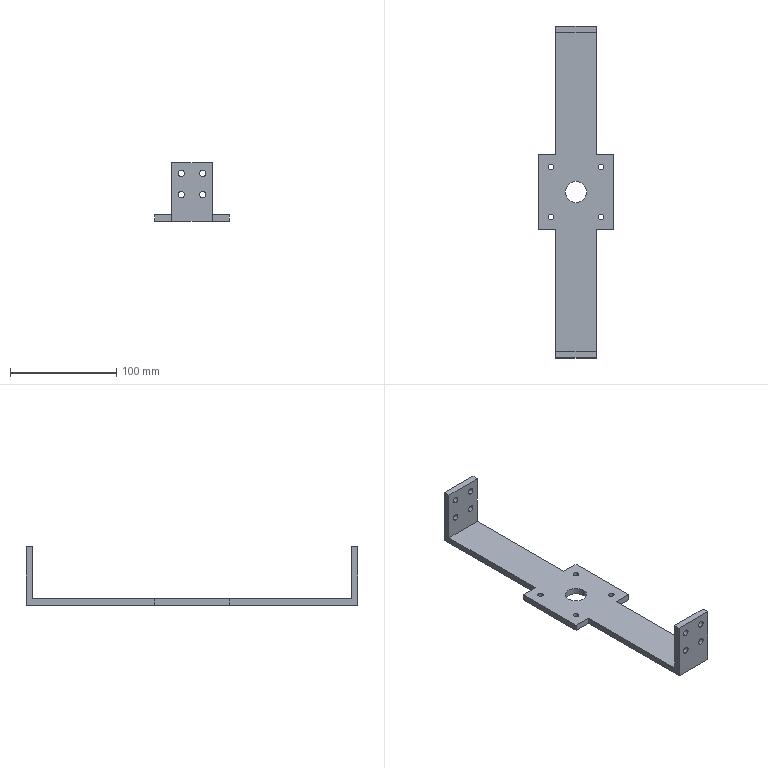Part | SolidWorks | features ICE 4, Cut 1, Extrusion 1 | 1 solid | 44 faces | box 70 x 312 x 55 mm | volume 103168 mm3 | cylinder 26 | plane 18 | commonest cylinder face diameters 6 x16 5.2 x8 20 x2
STEP:
#1=CARTESIAN_POINT('',(10.,156.,-21.5));
#2=VERTEX_POINT('',#1);
#3=CARTESIAN_POINT('',(-10.,156.,-21.5));
#4=VERTEX_POINT('',#3);
#5=CARTESIAN_POINT('',(0.,156.,-21.5));
#6=DIRECTION('',(0.,0.,-1.));
#7=DIRECTION('',(-1.,0.,0.));
#8=AXIS2_PLACEMENT_3D('',#5,#6,#7);
#9=CIRCLE('',#8,10.);
#10=EDGE_CURVE('',#2,#4,#9,.T.);
#11=ORIENTED_EDGE('',*,*,#10,.F.);
#12=CARTESIAN_POINT('',(10.,156.,-27.5));
#13=VERTEX_POINT('',#12);
#14=CARTESIAN_POINT('',(10.,156.,-17.5));
#15=DIRECTION('',(0.,0.,-1.));
#16=VECTOR('',#15,1000.);
#17=LINE('',#14,#16);
#18=EDGE_CURVE('',#2,#13,#17,.T.);
#19=ORIENTED_EDGE('',*,*,#18,.T.);
#20=CARTESIAN_POINT('',(-10.,156.,-27.5));
#21=VERTEX_POINT('',#20);
#22=CARTESIAN_POINT('',(0.,156.,-27.5));
#23=DIRECTION('',(0.,0.,-1.));
#24=DIRECTION('',(-1.,0.,0.));
#25=AXIS2_PLACEMENT_3D('',#22,#23,#24);
#26=CIRCLE('',#25,10.);
#27=EDGE_CURVE('',#13,#21,#26,.T.);
#28=ORIENTED_EDGE('',*,*,#27,.T.);
#29=CARTESIAN_POINT('',(-10.,156.,-17.5));
#30=DIRECTION('',(0.,0.,-1.));
#31=VECTOR('',#30,1000.);
#32=LINE('',#29,#31);
#33=EDGE_CURVE('',#4,#21,#32,.T.);
#34=ORIENTED_EDGE('',*,*,#33,.F.);
#35=EDGE_LOOP('',(#11,#19,#28,#34));
#36=FACE_OUTER_BOUND('',#35,.T.);
#37=CARTESIAN_POINT('',(0.,156.,-17.5));
#38=DIRECTION('',(0.,0.,-1.));
#39=DIRECTION('',(-1.,0.,0.));
#40=AXIS2_PLACEMENT_3D('',#37,#38,#39);
#41=CYLINDRICAL_SURFACE('',#40,10.);
#42=ADVANCED_FACE('',(#36),#41,.F.);
#43=CARTESIAN_POINT('',(26.145,179.545,-21.5));
#44=VERTEX_POINT('',#43);
#45=CARTESIAN_POINT('',(20.945,179.545,-21.5));
#46=VERTEX_POINT('',#45);
#47=CARTESIAN_POINT('',(23.545,179.545,-21.5));
#48=DIRECTION('',(0.,0.,-1.));
#49=DIRECTION('',(-1.,0.,0.));
#50=AXIS2_PLACEMENT_3D('',#47,#48,#49);
#51=CIRCLE('',#50,2.6);
#52=EDGE_CURVE('',#44,#46,#51,.T.);
#53=ORIENTED_EDGE('',*,*,#52,.F.);
#54=CARTESIAN_POINT('',(26.145,179.545,-27.5));
#55=VERTEX_POINT('',#54);
#56=CARTESIAN_POINT('',(26.145,179.545,-17.5));
#57=DIRECTION('',(0.,0.,-1.));
#58=VECTOR('',#57,1000.);
#59=LINE('',#56,#58);
#60=EDGE_CURVE('',#44,#55,#59,.T.);
#61=ORIENTED_EDGE('',*,*,#60,.T.);
#62=CARTESIAN_POINT('',(20.945,179.545,-27.5));
#63=VERTEX_POINT('',#62);
#64=CARTESIAN_POINT('',(23.545,179.545,-27.5));
#65=DIRECTION('',(0.,0.,-1.));
#66=DIRECTION('',(-1.,0.,0.));
#67=AXIS2_PLACEMENT_3D('',#64,#65,#66);
#68=CIRCLE('',#67,2.6);
#69=EDGE_CURVE('',#55,#63,#68,.T.);
#70=ORIENTED_EDGE('',*,*,#69,.T.);
#71=CARTESIAN_POINT('',(20.945,179.545,-17.5));
#72=DIRECTION('',(0.,0.,-1.));
#73=VECTOR('',#72,1000.);
#74=LINE('',#71,#73);
#75=EDGE_CURVE('',#46,#63,#74,.T.);
#76=ORIENTED_EDGE('',*,*,#75,.F.);
#77=EDGE_LOOP('',(#53,#61,#70,#76));
#78=FACE_OUTER_BOUND('',#77,.T.);
#79=CARTESIAN_POINT('',(23.545,179.545,-17.5));
#80=DIRECTION('',(0.,0.,-1.));
#81=DIRECTION('',(-1.,0.,0.));
#82=AXIS2_PLACEMENT_3D('',#79,#80,#81);
#83=CYLINDRICAL_SURFACE('',#82,2.6);
#84=ADVANCED_FACE('',(#78),#83,.F.);
#85=CARTESIAN_POINT('',(26.1,132.5,-21.5));
#86=VERTEX_POINT('',#85);
#87=CARTESIAN_POINT('',(20.9,132.5,-21.5));
#88=VERTEX_POINT('',#87);
#89=CARTESIAN_POINT('',(23.5,132.5,-21.5));
#90=DIRECTION('',(0.,0.,-1.));
#91=DIRECTION('',(-1.,0.,0.));
#92=AXIS2_PLACEMENT_3D('',#89,#90,#91);
#93=CIRCLE('',#92,2.6);
#94=EDGE_CURVE('',#86,#88,#93,.T.);
#95=ORIENTED_EDGE('',*,*,#94,.F.);
#96=CARTESIAN_POINT('',(26.1,132.5,-27.5));
#97=VERTEX_POINT('',#96);
#98=CARTESIAN_POINT('',(26.1,132.5,-17.5));
#99=DIRECTION('',(0.,0.,-1.));
#100=VECTOR('',#99,1000.);
#101=LINE('',#98,#100);
#102=EDGE_CURVE('',#86,#97,#101,.T.);
#103=ORIENTED_EDGE('',*,*,#102,.T.);
#104=CARTESIAN_POINT('',(20.9,132.5,-27.5));
#105=VERTEX_POINT('',#104);
#106=CARTESIAN_POINT('',(23.5,132.5,-27.5));
#107=DIRECTION('',(0.,0.,-1.));
#108=DIRECTION('',(-1.,0.,0.));
#109=AXIS2_PLACEMENT_3D('',#106,#107,#108);
#110=CIRCLE('',#109,2.6);
#111=EDGE_CURVE('',#97,#105,#110,.T.);
#112=ORIENTED_EDGE('',*,*,#111,.T.);
#113=CARTESIAN_POINT('',(20.9,132.5,-17.5));
#114=DIRECTION('',(0.,0.,-1.));
#115=VECTOR('',#114,1000.);
#116=LINE('',#113,#115);
#117=EDGE_CURVE('',#88,#105,#116,.T.);
#118=ORIENTED_EDGE('',*,*,#117,.F.);
#119=EDGE_LOOP('',(#95,#103,#112,#118));
#120=FACE_OUTER_BOUND('',#119,.T.);
#121=CARTESIAN_POINT('',(23.5,132.5,-17.5));
#122=DIRECTION('',(0.,0.,-1.));
#123=DIRECTION('',(-1.,0.,0.));
#124=AXIS2_PLACEMENT_3D('',#121,#122,#123);
#125=CYLINDRICAL_SURFACE('',#124,2.6);
#126=ADVANCED_FACE('',(#120),#125,.F.);
#127=CARTESIAN_POINT('',(-20.9,132.5,-21.5));
#128=VERTEX_POINT('',#127);
#129=CARTESIAN_POINT('',(-26.1,132.5,-21.5));
#130=VERTEX_POINT('',#129);
#131=CARTESIAN_POINT('',(-23.5,132.5,-21.5));
#132=DIRECTION('',(0.,0.,-1.));
#133=DIRECTION('',(-1.,0.,0.));
#134=AXIS2_PLACEMENT_3D('',#131,#132,#133);
#135=CIRCLE('',#134,2.6);
#136=EDGE_CURVE('',#128,#130,#135,.T.);
#137=ORIENTED_EDGE('',*,*,#136,.F.);
#138=CARTESIAN_POINT('',(-20.9,132.5,-27.5));
#139=VERTEX_POINT('',#138);
#140=CARTESIAN_POINT('',(-20.9,132.5,-17.5));
#141=DIRECTION('',(0.,0.,-1.));
#142=VECTOR('',#141,1000.);
#143=LINE('',#140,#142);
#144=EDGE_CURVE('',#128,#139,#143,.T.);
#145=ORIENTED_EDGE('',*,*,#144,.T.);
#146=CARTESIAN_POINT('',(-26.1,132.5,-27.5));
#147=VERTEX_POINT('',#146);
#148=CARTESIAN_POINT('',(-23.5,132.5,-27.5));
#149=DIRECTION('',(0.,0.,-1.));
#150=DIRECTION('',(-1.,0.,0.));
#151=AXIS2_PLACEMENT_3D('',#148,#149,#150);
#152=CIRCLE('',#151,2.6);
#153=EDGE_CURVE('',#139,#147,#152,.T.);
#154=ORIENTED_EDGE('',*,*,#153,.T.);
#155=CARTESIAN_POINT('',(-26.1,132.5,-17.5));
#156=DIRECTION('',(0.,0.,-1.));
#157=VECTOR('',#156,1000.);
#158=LINE('',#155,#157);
#159=EDGE_CURVE('',#130,#147,#158,.T.);
#160=ORIENTED_EDGE('',*,*,#159,.F.);
#161=EDGE_LOOP('',(#137,#145,#154,#160));
#162=FACE_OUTER_BOUND('',#161,.T.);
#163=CARTESIAN_POINT('',(-23.5,132.5,-17.5));
#164=DIRECTION('',(0.,0.,-1.));
#165=DIRECTION('',(-1.,0.,0.));
#166=AXIS2_PLACEMENT_3D('',#163,#164,#165);
#167=CYLINDRICAL_SURFACE('',#166,2.6);
#168=ADVANCED_FACE('',(#162),#167,.F.);
#169=CARTESIAN_POINT('',(-20.945,179.545,-21.5));
#170=VERTEX_POINT('',#169);
#171=CARTESIAN_POINT('',(-26.145,179.545,-21.5));
#172=VERTEX_POINT('',#171);
#173=CARTESIAN_POINT('',(-23.545,179.545,-21.5));
#174=DIRECTION('',(0.,0.,-1.));
#175=DIRECTION('',(-1.,0.,0.));
#176=AXIS2_PLACEMENT_3D('',#173,#174,#175);
#177=CIRCLE('',#176,2.6);
#178=EDGE_CURVE('',#170,#172,#177,.T.);
#179=ORIENTED_EDGE('',*,*,#178,.F.);
#180=CARTESIAN_POINT('',(-20.945,179.545,-27.5));
#181=VERTEX_POINT('',#180);
#182=CARTESIAN_POINT('',(-20.945,179.545,-17.5));
#183=DIRECTION('',(0.,0.,-1.));
#184=VECTOR('',#183,1000.);
#185=LINE('',#182,#184);
#186=EDGE_CURVE('',#170,#181,#185,.T.);
#187=ORIENTED_EDGE('',*,*,#186,.T.);
#188=CARTESIAN_POINT('',(-26.145,179.545,-27.5));
#189=VERTEX_POINT('',#188);
#190=CARTESIAN_POINT('',(-23.545,179.545,-27.5));
#191=DIRECTION('',(0.,0.,-1.));
#192=DIRECTION('',(-1.,0.,0.));
#193=AXIS2_PLACEMENT_3D('',#190,#191,#192);
#194=CIRCLE('',#193,2.6);
#195=EDGE_CURVE('',#181,#189,#194,.T.);
#196=ORIENTED_EDGE('',*,*,#195,.T.);
#197=CARTESIAN_POINT('',(-26.145,179.545,-17.5));
#198=DIRECTION('',(0.,0.,-1.));
#199=VECTOR('',#198,1000.);
#200=LINE('',#197,#199);
#201=EDGE_CURVE('',#172,#189,#200,.T.);
#202=ORIENTED_EDGE('',*,*,#201,.F.);
#203=EDGE_LOOP('',(#179,#187,#196,#202));
#204=FACE_OUTER_BOUND('',#203,.T.);
#205=CARTESIAN_POINT('',(-23.545,179.545,-17.5));
#206=DIRECTION('',(0.,0.,-1.));
#207=DIRECTION('',(-1.,0.,0.));
#208=AXIS2_PLACEMENT_3D('',#205,#206,#207);
#209=CYLINDRICAL_SURFACE('',#208,2.6);
#210=ADVANCED_FACE('',(#204),#209,.F.);
#211=CARTESIAN_POINT('',(10.,312.,14.5));
#212=VERTEX_POINT('',#211);
#213=CARTESIAN_POINT('',(10.,312.,20.5));
#214=VERTEX_POINT('',#213);
#215=CARTESIAN_POINT('',(10.,312.,17.5));
#216=DIRECTION('',(0.,1.,0.));
#217=DIRECTION('',(0.,0.,1.));
#218=AXIS2_PLACEMENT_3D('',#215,#216,#217);
#219=CIRCLE('',#218,3.);
#220=EDGE_CURVE('',#212,#214,#219,.T.);
#221=ORIENTED_EDGE('',*,*,#220,.T.);
#222=CARTESIAN_POINT('',(10.,306.,20.5));
#223=VERTEX_POINT('',#222);
#224=CARTESIAN_POINT('',(10.,312.,20.5));
#225=DIRECTION('',(0.,-1.,0.));
#226=VECTOR('',#225,1000.);
#227=LINE('',#224,#226);
#228=EDGE_CURVE('',#214,#223,#227,.T.);
#229=ORIENTED_EDGE('',*,*,#228,.T.);
#230=CARTESIAN_POINT('',(10.,306.,14.5));
#231=VERTEX_POINT('',#230);
#232=CARTESIAN_POINT('',(10.,306.,17.5));
#233=DIRECTION('',(0.,1.,0.));
#234=DIRECTION('',(0.,0.,1.));
#235=AXIS2_PLACEMENT_3D('',#232,#233,#234);
#236=CIRCLE('',#235,3.);
#237=EDGE_CURVE('',#231,#223,#236,.T.);
#238=ORIENTED_EDGE('',*,*,#237,.F.);
#239=CARTESIAN_POINT('',(10.,312.,14.5));
#240=DIRECTION('',(0.,-1.,0.));
#241=VECTOR('',#240,1000.);
#242=LINE('',#239,#241);
#243=EDGE_CURVE('',#212,#231,#242,.T.);
#244=ORIENTED_EDGE('',*,*,#243,.F.);
#245=EDGE_LOOP('',(#221,#229,#238,#244));
#246=FACE_OUTER_BOUND('',#245,.T.);
#247=CARTESIAN_POINT('',(10.,312.,17.5));
#248=DIRECTION('',(0.,-1.,0.));
#249=DIRECTION('',(0.,0.,-1.));
#250=AXIS2_PLACEMENT_3D('',#247,#248,#249);
#251=CYLINDRICAL_SURFACE('',#250,3.);
#252=ADVANCED_FACE('',(#246),#251,.F.);
#253=CARTESIAN_POINT('',(-10.,312.,14.5));
#254=VERTEX_POINT('',#253);
#255=CARTESIAN_POINT('',(-10.,312.,20.5));
#256=VERTEX_POINT('',#255);
#257=CARTESIAN_POINT('',(-10.,312.,17.5));
#258=DIRECTION('',(0.,1.,0.));
#259=DIRECTION('',(0.,0.,1.));
#260=AXIS2_PLACEMENT_3D('',#257,#258,#259);
#261=CIRCLE('',#260,3.);
#262=EDGE_CURVE('',#254,#256,#261,.T.);
#263=ORIENTED_EDGE('',*,*,#262,.T.);
#264=CARTESIAN_POINT('',(-10.,306.,20.5));
#265=VERTEX_POINT('',#264);
#266=CARTESIAN_POINT('',(-10.,312.,20.5));
#267=DIRECTION('',(0.,-1.,0.));
#268=VECTOR('',#267,1000.);
#269=LINE('',#266,#268);
#270=EDGE_CURVE('',#256,#265,#269,.T.);
#271=ORIENTED_EDGE('',*,*,#270,.T.);
#272=CARTESIAN_POINT('',(-10.,306.,14.5));
#273=VERTEX_POINT('',#272);
#274=CARTESIAN_POINT('',(-10.,306.,17.5));
#275=DIRECTION('',(0.,1.,0.));
#276=DIRECTION('',(0.,0.,1.));
#277=AXIS2_PLACEMENT_3D('',#274,#275,#276);
#278=CIRCLE('',#277,3.);
#279=EDGE_CURVE('',#273,#265,#278,.T.);
#280=ORIENTED_EDGE('',*,*,#279,.F.);
#281=CARTESIAN_POINT('',(-10.,312.,14.5));
#282=DIRECTION('',(0.,-1.,0.));
#283=VECTOR('',#282,1000.);
#284=LINE('',#281,#283);
#285=EDGE_CURVE('',#254,#273,#284,.T.);
#286=ORIENTED_EDGE('',*,*,#285,.F.);
#287=EDGE_LOOP('',(#263,#271,#280,#286));
#288=FACE_OUTER_BOUND('',#287,.T.);
#289=CARTESIAN_POINT('',(-10.,312.,17.5));
#290=DIRECTION('',(0.,-1.,0.));
#291=DIRECTION('',(0.,0.,-1.));
#292=AXIS2_PLACEMENT_3D('',#289,#290,#291);
#293=CYLINDRICAL_SURFACE('',#292,3.);
#294=ADVANCED_FACE('',(#288),#293,.F.);
#295=CARTESIAN_POINT('',(10.,312.,-5.5));
#296=VERTEX_POINT('',#295);
#297=CARTESIAN_POINT('',(10.,312.,0.5));
#298=VERTEX_POINT('',#297);
#299=CARTESIAN_POINT('',(10.,312.,-2.5));
#300=DIRECTION('',(0.,1.,0.));
#301=DIRECTION('',(0.,0.,1.));
#302=AXIS2_PLACEMENT_3D('',#299,#300,#301);
#303=CIRCLE('',#302,3.);
#304=EDGE_CURVE('',#296,#298,#303,.T.);
#305=ORIENTED_EDGE('',*,*,#304,.T.);
#306=CARTESIAN_POINT('',(10.,306.,0.5));
#307=VERTEX_POINT('',#306);
#308=CARTESIAN_POINT('',(10.,312.,0.5));
#309=DIRECTION('',(0.,-1.,0.));
#310=VECTOR('',#309,1000.);
#311=LINE('',#308,#310);
#312=EDGE_CURVE('',#298,#307,#311,.T.);
#313=ORIENTED_EDGE('',*,*,#312,.T.);
#314=CARTESIAN_POINT('',(10.,306.,-5.5));
#315=VERTEX_POINT('',#314);
#316=CARTESIAN_POINT('',(10.,306.,-2.5));
#317=DIRECTION('',(0.,1.,0.));
#318=DIRECTION('',(0.,0.,1.));
#319=AXIS2_PLACEMENT_3D('',#316,#317,#318);
#320=CIRCLE('',#319,3.);
#321=EDGE_CURVE('',#315,#307,#320,.T.);
#322=ORIENTED_EDGE('',*,*,#321,.F.);
#323=CARTESIAN_POINT('',(10.,312.,-5.5));
#324=DIRECTION('',(0.,-1.,0.));
#325=VECTOR('',#324,1000.);
#326=LINE('',#323,#325);
#327=EDGE_CURVE('',#296,#315,#326,.T.);
#328=ORIENTED_EDGE('',*,*,#327,.F.);
#329=EDGE_LOOP('',(#305,#313,#322,#328));
#330=FACE_OUTER_BOUND('',#329,.T.);
#331=CARTESIAN_POINT('',(10.,312.,-2.5));
#332=DIRECTION('',(0.,-1.,0.));
#333=DIRECTION('',(0.,0.,-1.));
#334=AXIS2_PLACEMENT_3D('',#331,#332,#333);
#335=CYLINDRICAL_SURFACE('',#334,3.);
#336=ADVANCED_FACE('',(#330),#335,.F.);
#337=CARTESIAN_POINT('',(-10.,312.,-5.5));
#338=VERTEX_POINT('',#337);
#339=CARTESIAN_POINT('',(-10.,312.,0.5));
#340=VERTEX_POINT('',#339);
#341=CARTESIAN_POINT('',(-10.,312.,-2.5));
#342=DIRECTION('',(0.,1.,0.));
#343=DIRECTION('',(0.,0.,1.));
#344=AXIS2_PLACEMENT_3D('',#341,#342,#343);
#345=CIRCLE('',#344,3.);
#346=EDGE_CURVE('',#338,#340,#345,.T.);
#347=ORIENTED_EDGE('',*,*,#346,.T.);
#348=CARTESIAN_POINT('',(-10.,306.,0.5));
#349=VERTEX_POINT('',#348);
#350=CARTESIAN_POINT('',(-10.,312.,0.5));
#351=DIRECTION('',(0.,-1.,0.));
#352=VECTOR('',#351,1000.);
#353=LINE('',#350,#352);
#354=EDGE_CURVE('',#340,#349,#353,.T.);
#355=ORIENTED_EDGE('',*,*,#354,.T.);
#356=CARTESIAN_POINT('',(-10.,306.,-5.5));
#357=VERTEX_POINT('',#356);
#358=CARTESIAN_POINT('',(-10.,306.,-2.5));
#359=DIRECTION('',(0.,1.,0.));
#360=DIRECTION('',(0.,0.,1.));
#361=AXIS2_PLACEMENT_3D('',#358,#359,#360);
#362=CIRCLE('',#361,3.);
#363=EDGE_CURVE('',#357,#349,#362,.T.);
#364=ORIENTED_EDGE('',*,*,#363,.F.);
#365=CARTESIAN_POINT('',(-10.,312.,-5.5));
#366=DIRECTION('',(0.,-1.,0.));
#367=VECTOR('',#366,1000.);
#368=LINE('',#365,#367);
#369=EDGE_CURVE('',#338,#357,#368,.T.);
#370=ORIENTED_EDGE('',*,*,#369,.F.);
#371=EDGE_LOOP('',(#347,#355,#364,#370));
#372=FACE_OUTER_BOUND('',#371,.T.);
#373=CARTESIAN_POINT('',(-10.,312.,-2.5));
#374=DIRECTION('',(0.,-1.,0.));
#375=DIRECTION('',(0.,0.,-1.));
#376=AXIS2_PLACEMENT_3D('',#373,#374,#375);
#377=CYLINDRICAL_SURFACE('',#376,3.);
#378=ADVANCED_FACE('',(#372),#377,.F.);
#379=CARTESIAN_POINT('',(-10.,0.,14.5));
#380=VERTEX_POINT('',#379);
#381=CARTESIAN_POINT('',(-10.,0.,20.5));
#382=VERTEX_POINT('',#381);
#383=CARTESIAN_POINT('',(-10.,0.,17.5));
#384=DIRECTION('',(0.,1.,0.));
#385=DIRECTION('',(0.,0.,1.));
#386=AXIS2_PLACEMENT_3D('',#383,#384,#385);
#387=CIRCLE('',#386,3.);
#388=EDGE_CURVE('',#380,#382,#387,.T.);
#389=ORIENTED_EDGE('',*,*,#388,.F.);
#390=CARTESIAN_POINT('',(-10.,6.,14.5));
#391=VERTEX_POINT('',#390);
#392=CARTESIAN_POINT('',(-10.,-10.,14.5));
#393=DIRECTION('',(0.,1.,0.));
#394=VECTOR('',#393,1000.);
#395=LINE('',#392,#394);
#396=EDGE_CURVE('',#380,#391,#395,.T.);
#397=ORIENTED_EDGE('',*,*,#396,.T.);
#398=CARTESIAN_POINT('',(-10.,6.,20.5));
#399=VERTEX_POINT('',#398);
#400=CARTESIAN_POINT('',(-10.,6.,17.5));
#401=DIRECTION('',(0.,1.,0.));
#402=DIRECTION('',(0.,0.,1.));
#403=AXIS2_PLACEMENT_3D('',#400,#401,#402);
#404=CIRCLE('',#403,3.);
#405=EDGE_CURVE('',#391,#399,#404,.T.);
#406=ORIENTED_EDGE('',*,*,#405,.T.);
#407=CARTESIAN_POINT('',(-10.,-10.,20.5));
#408=DIRECTION('',(0.,1.,0.));
#409=VECTOR('',#408,1000.);
#410=LINE('',#407,#409);
#411=EDGE_CURVE('',#382,#399,#410,.T.);
#412=ORIENTED_EDGE('',*,*,#411,.F.);
#413=EDGE_LOOP('',(#389,#397,#406,#412));
#414=FACE_OUTER_BOUND('',#413,.T.);
#415=CARTESIAN_POINT('',(-10.,-10.,17.5));
#416=DIRECTION('',(0.,1.,0.));
#417=DIRECTION('',(0.,0.,1.));
#418=AXIS2_PLACEMENT_3D('',#415,#416,#417);
#419=CYLINDRICAL_SURFACE('',#418,3.);
#420=ADVANCED_FACE('',(#414),#419,.F.);
#421=CARTESIAN_POINT('',(10.,0.,14.5));
#422=VERTEX_POINT('',#421);
#423=CARTESIAN_POINT('',(10.,0.,20.5));
#424=VERTEX_POINT('',#423);
#425=CARTESIAN_POINT('',(10.,0.,17.5));
#426=DIRECTION('',(0.,1.,0.));
#427=DIRECTION('',(0.,0.,1.));
#428=AXIS2_PLACEMENT_3D('',#425,#426,#427);
#429=CIRCLE('',#428,3.);
#430=EDGE_CURVE('',#422,#424,#429,.T.);
#431=ORIENTED_EDGE('',*,*,#430,.F.);
#432=CARTESIAN_POINT('',(10.,6.,14.5));
#433=VERTEX_POINT('',#432);
#434=CARTESIAN_POINT('',(10.,-10.,14.5));
#435=DIRECTION('',(0.,1.,0.));
#436=VECTOR('',#435,1000.);
#437=LINE('',#434,#436);
#438=EDGE_CURVE('',#422,#433,#437,.T.);
#439=ORIENTED_EDGE('',*,*,#438,.T.);
#440=CARTESIAN_POINT('',(10.,6.,20.5));
#441=VERTEX_POINT('',#440);
#442=CARTESIAN_POINT('',(10.,6.,17.5));
#443=DIRECTION('',(0.,1.,0.));
#444=DIRECTION('',(0.,0.,1.));
#445=AXIS2_PLACEMENT_3D('',#442,#443,#444);
#446=CIRCLE('',#445,3.);
#447=EDGE_CURVE('',#433,#441,#446,.T.);
#448=ORIENTED_EDGE('',*,*,#447,.T.);
#449=CARTESIAN_POINT('',(10.,-10.,20.5));
#450=DIRECTION('',(0.,1.,0.));
#451=VECTOR('',#450,1000.);
#452=LINE('',#449,#451);
#453=EDGE_CURVE('',#424,#441,#452,.T.);
#454=ORIENTED_EDGE('',*,*,#453,.F.);
#455=EDGE_LOOP('',(#431,#439,#448,#454));
#456=FACE_OUTER_BOUND('',#455,.T.);
#457=CARTESIAN_POINT('',(10.,-10.,17.5));
#458=DIRECTION('',(0.,1.,0.));
#459=DIRECTION('',(0.,0.,1.));
#460=AXIS2_PLACEMENT_3D('',#457,#458,#459);
#461=CYLINDRICAL_SURFACE('',#460,3.);
#462=ADVANCED_FACE('',(#456),#461,.F.);
#463=CARTESIAN_POINT('',(10.,0.,-5.5));
#464=VERTEX_POINT('',#463);
#465=CARTESIAN_POINT('',(10.,0.,0.5));
#466=VERTEX_POINT('',#465);
#467=CARTESIAN_POINT('',(10.,0.,-2.5));
#468=DIRECTION('',(0.,1.,0.));
#469=DIRECTION('',(0.,0.,1.));
#470=AXIS2_PLACEMENT_3D('',#467,#468,#469);
#471=CIRCLE('',#470,3.);
#472=EDGE_CURVE('',#464,#466,#471,.T.);
#473=ORIENTED_EDGE('',*,*,#472,.F.);
#474=CARTESIAN_POINT('',(10.,6.,-5.5));
#475=VERTEX_POINT('',#474);
#476=CARTESIAN_POINT('',(10.,-10.,-5.5));
#477=DIRECTION('',(0.,1.,0.));
#478=VECTOR('',#477,1000.);
#479=LINE('',#476,#478);
#480=EDGE_CURVE('',#464,#475,#479,.T.);
#481=ORIENTED_EDGE('',*,*,#480,.T.);
#482=CARTESIAN_POINT('',(10.,6.,0.5));
#483=VERTEX_POINT('',#482);
#484=CARTESIAN_POINT('',(10.,6.,-2.5));
#485=DIRECTION('',(0.,1.,0.));
#486=DIRECTION('',(0.,0.,1.));
#487=AXIS2_PLACEMENT_3D('',#484,#485,#486);
#488=CIRCLE('',#487,3.);
#489=EDGE_CURVE('',#475,#483,#488,.T.);
#490=ORIENTED_EDGE('',*,*,#489,.T.);
#491=CARTESIAN_POINT('',(10.,-10.,0.5));
#492=DIRECTION('',(0.,1.,0.));
#493=VECTOR('',#492,1000.);
#494=LINE('',#491,#493);
#495=EDGE_CURVE('',#466,#483,#494,.T.);
#496=ORIENTED_EDGE('',*,*,#495,.F.);
#497=EDGE_LOOP('',(#473,#481,#490,#496));
#498=FACE_OUTER_BOUND('',#497,.T.);
#499=CARTESIAN_POINT('',(10.,-10.,-2.5));
#500=DIRECTION('',(0.,1.,0.));
#501=DIRECTION('',(0.,0.,1.));
#502=AXIS2_PLACEMENT_3D('',#499,#500,#501);
#503=CYLINDRICAL_SURFACE('',#502,3.);
#504=ADVANCED_FACE('',(#498),#503,.F.);
#505=CARTESIAN_POINT('',(-10.,0.,-5.5));
#506=VERTEX_POINT('',#505);
#507=CARTESIAN_POINT('',(-10.,0.,0.5));
#508=VERTEX_POINT('',#507);
#509=CARTESIAN_POINT('',(-10.,0.,-2.5));
#510=DIRECTION('',(0.,1.,0.));
#511=DIRECTION('',(0.,0.,1.));
#512=AXIS2_PLACEMENT_3D('',#509,#510,#511);
#513=CIRCLE('',#512,3.);
#514=EDGE_CURVE('',#506,#508,#513,.T.);
#515=ORIENTED_EDGE('',*,*,#514,.F.);
#516=CARTESIAN_POINT('',(-10.,6.,-5.5));
#517=VERTEX_POINT('',#516);
#518=CARTESIAN_POINT('',(-10.,-10.,-5.5));
#519=DIRECTION('',(0.,1.,0.));
#520=VECTOR('',#519,1000.);
#521=LINE('',#518,#520);
#522=EDGE_CURVE('',#506,#517,#521,.T.);
#523=ORIENTED_EDGE('',*,*,#522,.T.);
#524=CARTESIAN_POINT('',(-10.,6.,0.5));
#525=VERTEX_POINT('',#524);
#526=CARTESIAN_POINT('',(-10.,6.,-2.5));
#527=DIRECTION('',(0.,1.,0.));
#528=DIRECTION('',(0.,0.,1.));
#529=AXIS2_PLACEMENT_3D('',#526,#527,#528);
#530=CIRCLE('',#529,3.);
#531=EDGE_CURVE('',#517,#525,#530,.T.);
#532=ORIENTED_EDGE('',*,*,#531,.T.);
#533=CARTESIAN_POINT('',(-10.,-10.,0.5));
#534=DIRECTION('',(0.,1.,0.));
#535=VECTOR('',#534,1000.);
#536=LINE('',#533,#535);
#537=EDGE_CURVE('',#508,#525,#536,.T.);
#538=ORIENTED_EDGE('',*,*,#537,.F.);
#539=EDGE_LOOP('',(#515,#523,#532,#538));
#540=FACE_OUTER_BOUND('',#539,.T.);
#541=CARTESIAN_POINT('',(-10.,-10.,-2.5));
#542=DIRECTION('',(0.,1.,0.));
#543=DIRECTION('',(0.,0.,1.));
#544=AXIS2_PLACEMENT_3D('',#541,#542,#543);
#545=CYLINDRICAL_SURFACE('',#544,3.);
#546=ADVANCED_FACE('',(#540),#545,.F.);
#547=CARTESIAN_POINT('',(19.,121.,-27.5));
#548=VERTEX_POINT('',#547);
#549=CARTESIAN_POINT('',(19.,0.,-27.5));
#550=VERTEX_POINT('',#549);
#551=CARTESIAN_POINT('',(19.,6.,-27.5));
#552=DIRECTION('',(0.,-1.,0.));
#553=VECTOR('',#552,1000.);
#554=LINE('',#551,#553);
#555=EDGE_CURVE('',#548,#550,#554,.T.);
#556=ORIENTED_EDGE('',*,*,#555,.F.);
#557=CARTESIAN_POINT('',(19.,121.,-21.5));
#558=VERTEX_POINT('',#557);
#559=CARTESIAN_POINT('',(19.,121.,-27.5));
#560=DIRECTION('',(0.,0.,1.));
#561=VECTOR('',#560,1000.);
#562=LINE('',#559,#561);
#563=EDGE_CURVE('',#548,#558,#562,.T.);
#564=ORIENTED_EDGE('',*,*,#563,.T.);
#565=CARTESIAN_POINT('',(19.,6.,-21.5));
#566=VERTEX_POINT('',#565);
#567=CARTESIAN_POINT('',(19.,306.,-21.5));
#568=DIRECTION('',(0.,-1.,0.));
#569=VECTOR('',#568,1000.);
#570=LINE('',#567,#569);
#571=EDGE_CURVE('',#558,#566,#570,.T.);
#572=ORIENTED_EDGE('',*,*,#571,.T.);
#573=CARTESIAN_POINT('',(19.,6.,27.5));
#574=VERTEX_POINT('',#573);
#575=CARTESIAN_POINT('',(19.,6.,-27.5));
#576=DIRECTION('',(0.,0.,-1.));
#577=VECTOR('',#576,1000.);
#578=LINE('',#575,#577);
#579=EDGE_CURVE('',#574,#566,#578,.T.);
#580=ORIENTED_EDGE('',*,*,#579,.F.);
#581=CARTESIAN_POINT('',(19.,0.,27.5));
#582=VERTEX_POINT('',#581);
#583=CARTESIAN_POINT('',(19.,6.,27.5));
#584=DIRECTION('',(0.,-1.,0.));
#585=VECTOR('',#584,1000.);
#586=LINE('',#583,#585);
#587=EDGE_CURVE('',#574,#582,#586,.T.);
#588=ORIENTED_EDGE('',*,*,#587,.T.);
#589=CARTESIAN_POINT('',(19.,0.,-27.5));
#590=DIRECTION('',(0.,0.,-1.));
#591=VECTOR('',#590,1000.);
#592=LINE('',#589,#591);
#593=EDGE_CURVE('',#582,#550,#592,.T.);
#594=ORIENTED_EDGE('',*,*,#593,.T.);
#595=EDGE_LOOP('',(#556,#564,#572,#580,#588,#594));
#596=FACE_OUTER_BOUND('',#595,.T.);
#597=CARTESIAN_POINT('',(19.,6.,-27.5));
#598=DIRECTION('',(-1.,0.,0.));
#599=DIRECTION('',(0.,0.,1.));
#600=AXIS2_PLACEMENT_3D('',#597,#598,#599);
#601=PLANE('',#600);
#602=ADVANCED_FACE('',(#596),#601,.F.);
#603=CARTESIAN_POINT('',(-19.,121.,-21.5));
#604=VERTEX_POINT('',#603);
#605=CARTESIAN_POINT('',(-19.,6.,-21.5));
#606=VERTEX_POINT('',#605);
#607=CARTESIAN_POINT('',(-19.,306.,-21.5));
#608=DIRECTION('',(0.,-1.,0.));
#609=VECTOR('',#608,1000.);
#610=LINE('',#607,#609);
#611=EDGE_CURVE('',#604,#606,#610,.T.);
#612=ORIENTED_EDGE('',*,*,#611,.F.);
#613=CARTESIAN_POINT('',(-19.,121.,-27.5));
#614=VERTEX_POINT('',#613);
#615=CARTESIAN_POINT('',(-19.,121.,-27.5));
#616=DIRECTION('',(0.,0.,-1.));
#617=VECTOR('',#616,1000.);
#618=LINE('',#615,#617);
#619=EDGE_CURVE('',#604,#614,#618,.T.);
#620=ORIENTED_EDGE('',*,*,#619,.T.);
#621=CARTESIAN_POINT('',(-19.,0.,-27.5));
#622=VERTEX_POINT('',#621);
#623=CARTESIAN_POINT('',(-19.,6.,-27.5));
#624=DIRECTION('',(0.,-1.,0.));
#625=VECTOR('',#624,1000.);
#626=LINE('',#623,#625);
#627=EDGE_CURVE('',#614,#622,#626,.T.);
#628=ORIENTED_EDGE('',*,*,#627,.T.);
#629=CARTESIAN_POINT('',(-19.,0.,27.5));
#630=VERTEX_POINT('',#629);
#631=CARTESIAN_POINT('',(-19.,0.,-27.5));
#632=DIRECTION('',(0.,0.,1.));
#633=VECTOR('',#632,1000.);
#634=LINE('',#631,#633);
#635=EDGE_CURVE('',#622,#630,#634,.T.);
#636=ORIENTED_EDGE('',*,*,#635,.T.);
#637=CARTESIAN_POINT('',(-19.,6.,27.5));
#638=VERTEX_POINT('',#637);
#639=CARTESIAN_POINT('',(-19.,6.,27.5));
#640=DIRECTION('',(0.,-1.,0.));
#641=VECTOR('',#640,1000.);
#642=LINE('',#639,#641);
#643=EDGE_CURVE('',#638,#630,#642,.T.);
#644=ORIENTED_EDGE('',*,*,#643,.F.);
#645=CARTESIAN_POINT('',(-19.,6.,-27.5));
#646=DIRECTION('',(0.,0.,1.));
#647=VECTOR('',#646,1000.);
#648=LINE('',#645,#647);
#649=EDGE_CURVE('',#606,#638,#648,.T.);
#650=ORIENTED_EDGE('',*,*,#649,.F.);
#651=EDGE_LOOP('',(#612,#620,#628,#636,#644,#650));
#652=FACE_OUTER_BOUND('',#651,.T.);
#653=CARTESIAN_POINT('',(-19.,6.,-27.5));
#654=DIRECTION('',(1.,0.,0.));
#655=DIRECTION('',(0.,0.,-1.));
#656=AXIS2_PLACEMENT_3D('',#653,#654,#655);
#657=PLANE('',#656);
#658=ADVANCED_FACE('',(#652),#657,.F.);
#659=CARTESIAN_POINT('',(19.,306.,-21.5));
#660=VERTEX_POINT('',#659);
#661=CARTESIAN_POINT('',(19.,191.,-21.5));
#662=VERTEX_POINT('',#661);
#663=CARTESIAN_POINT('',(19.,306.,-21.5));
#664=DIRECTION('',(0.,-1.,0.));
#665=VECTOR('',#664,1000.);
#666=LINE('',#663,#665);
#667=EDGE_CURVE('',#660,#662,#666,.T.);
#668=ORIENTED_EDGE('',*,*,#667,.T.);
#669=CARTESIAN_POINT('',(19.,191.,-27.5));
#670=VERTEX_POINT('',#669);
#671=CARTESIAN_POINT('',(19.,191.,-27.5));
#672=DIRECTION('',(0.,0.,-1.));
#673=VECTOR('',#672,1000.);
#674=LINE('',#671,#673);
#675=EDGE_CURVE('',#662,#670,#674,.T.);
#676=ORIENTED_EDGE('',*,*,#675,.T.);
#677=CARTESIAN_POINT('',(19.,312.,-27.5));
#678=VERTEX_POINT('',#677);
#679=CARTESIAN_POINT('',(19.,6.,-27.5));
#680=DIRECTION('',(0.,-1.,0.));
#681=VECTOR('',#680,1000.);
#682=LINE('',#679,#681);
#683=EDGE_CURVE('',#678,#670,#682,.T.);
#684=ORIENTED_EDGE('',*,*,#683,.F.);
#685=CARTESIAN_POINT('',(19.,312.,27.5));
#686=VERTEX_POINT('',#685);
#687=CARTESIAN_POINT('',(19.,312.,27.5));
#688=DIRECTION('',(0.,0.,-1.));
#689=VECTOR('',#688,1000.);
#690=LINE('',#687,#689);
#691=EDGE_CURVE('',#686,#678,#690,.T.);
#692=ORIENTED_EDGE('',*,*,#691,.F.);
#693=CARTESIAN_POINT('',(19.,306.,27.5));
#694=VERTEX_POINT('',#693);
#695=CARTESIAN_POINT('',(19.,312.,27.5));
#696=DIRECTION('',(0.,-1.,0.));
#697=VECTOR('',#696,1000.);
#698=LINE('',#695,#697);
#699=EDGE_CURVE('',#686,#694,#698,.T.);
#700=ORIENTED_EDGE('',*,*,#699,.T.);
#701=CARTESIAN_POINT('',(19.,306.,-21.5));
#702=DIRECTION('',(0.,0.,-1.));
#703=VECTOR('',#702,1000.);
#704=LINE('',#701,#703);
#705=EDGE_CURVE('',#694,#660,#704,.T.);
#706=ORIENTED_EDGE('',*,*,#705,.T.);
#707=EDGE_LOOP('',(#668,#676,#684,#692,#700,#706));
#708=FACE_OUTER_BOUND('',#707,.T.);
#709=CARTESIAN_POINT('',(19.,6.,-27.5));
#710=DIRECTION('',(-1.,0.,0.));
#711=DIRECTION('',(0.,0.,1.));
#712=AXIS2_PLACEMENT_3D('',#709,#710,#711);
#713=PLANE('',#712);
#714=ADVANCED_FACE('',(#708),#713,.F.);
#715=CARTESIAN_POINT('',(0.,156.,-27.5));
#716=DIRECTION('',(0.,0.,-1.));
#717=DIRECTION('',(-1.,0.,0.));
#718=AXIS2_PLACEMENT_3D('',#715,#716,#717);
#719=CIRCLE('',#718,10.);
#720=EDGE_CURVE('',#21,#13,#719,.T.);
#721=ORIENTED_EDGE('',*,*,#720,.F.);
#722=ORIENTED_EDGE('',*,*,#27,.F.);
#723=EDGE_LOOP('',(#721,#722));
#724=FACE_BOUND('',#723,.T.);
#725=CARTESIAN_POINT('',(23.545,179.545,-27.5));
#726=DIRECTION('',(0.,0.,-1.));
#727=DIRECTION('',(-1.,0.,0.));
#728=AXIS2_PLACEMENT_3D('',#725,#726,#727);
#729=CIRCLE('',#728,2.6);
#730=EDGE_CURVE('',#63,#55,#729,.T.);
#731=ORIENTED_EDGE('',*,*,#730,.F.);
#732=ORIENTED_EDGE('',*,*,#69,.F.);
#733=EDGE_LOOP('',(#731,#732));
#734=FACE_BOUND('',#733,.T.);
#735=CARTESIAN_POINT('',(23.5,132.5,-27.5));
#736=DIRECTION('',(0.,0.,-1.));
#737=DIRECTION('',(-1.,0.,0.));
#738=AXIS2_PLACEMENT_3D('',#735,#736,#737);
#739=CIRCLE('',#738,2.6);
#740=EDGE_CURVE('',#105,#97,#739,.T.);
#741=ORIENTED_EDGE('',*,*,#740,.F.);
#742=ORIENTED_EDGE('',*,*,#111,.F.);
#743=EDGE_LOOP('',(#741,#742));
#744=FACE_BOUND('',#743,.T.);
#745=CARTESIAN_POINT('',(-23.5,132.5,-27.5));
#746=DIRECTION('',(0.,0.,-1.));
#747=DIRECTION('',(-1.,0.,0.));
#748=AXIS2_PLACEMENT_3D('',#745,#746,#747);
#749=CIRCLE('',#748,2.6);
#750=EDGE_CURVE('',#147,#139,#749,.T.);
#751=ORIENTED_EDGE('',*,*,#750,.F.);
#752=ORIENTED_EDGE('',*,*,#153,.F.);
#753=EDGE_LOOP('',(#751,#752));
#754=FACE_BOUND('',#753,.T.);
#755=CARTESIAN_POINT('',(-23.545,179.545,-27.5));
#756=DIRECTION('',(0.,0.,-1.));
#757=DIRECTION('',(-1.,0.,0.));
#758=AXIS2_PLACEMENT_3D('',#755,#756,#757);
#759=CIRCLE('',#758,2.6);
#760=EDGE_CURVE('',#189,#181,#759,.T.);
#761=ORIENTED_EDGE('',*,*,#760,.F.);
#762=ORIENTED_EDGE('',*,*,#195,.F.);
#763=EDGE_LOOP('',(#761,#762));
#764=FACE_BOUND('',#763,.T.);
#765=ORIENTED_EDGE('',*,*,#683,.T.);
#766=CARTESIAN_POINT('',(35.,191.,-27.5));
#767=VERTEX_POINT('',#766);
#768=CARTESIAN_POINT('',(35.,191.,-27.5));
#769=DIRECTION('',(1.,0.,0.));
#770=VECTOR('',#769,1000.);
#771=LINE('',#768,#770);
#772=EDGE_CURVE('',#670,#767,#771,.T.);
#773=ORIENTED_EDGE('',*,*,#772,.T.);
#774=CARTESIAN_POINT('',(35.,121.,-27.5));
#775=VERTEX_POINT('',#774);
#776=CARTESIAN_POINT('',(35.,121.,-27.5));
#777=DIRECTION('',(0.,-1.,0.));
#778=VECTOR('',#777,1000.);
#779=LINE('',#776,#778);
#780=EDGE_CURVE('',#767,#775,#779,.T.);
#781=ORIENTED_EDGE('',*,*,#780,.T.);
#782=CARTESIAN_POINT('',(35.,121.,-27.5));
#783=DIRECTION('',(-1.,0.,0.));
#784=VECTOR('',#783,1000.);
#785=LINE('',#782,#784);
#786=EDGE_CURVE('',#775,#548,#785,.T.);
#787=ORIENTED_EDGE('',*,*,#786,.T.);
#788=ORIENTED_EDGE('',*,*,#555,.T.);
#789=CARTESIAN_POINT('',(-19.,0.,-27.5));
#790=DIRECTION('',(-1.,0.,0.));
#791=VECTOR('',#790,1000.);
#792=LINE('',#789,#791);
#793=EDGE_CURVE('',#550,#622,#792,.T.);
#794=ORIENTED_EDGE('',*,*,#793,.T.);
#795=ORIENTED_EDGE('',*,*,#627,.F.);
#796=CARTESIAN_POINT('',(-35.,121.,-27.5));
#797=VERTEX_POINT('',#796);
#798=CARTESIAN_POINT('',(35.,121.,-27.5));
#799=DIRECTION('',(-1.,0.,0.));
#800=VECTOR('',#799,1000.);
#801=LINE('',#798,#800);
#802=EDGE_CURVE('',#614,#797,#801,.T.);
#803=ORIENTED_EDGE('',*,*,#802,.T.);
#804=CARTESIAN_POINT('',(-35.,191.,-27.5));
#805=VERTEX_POINT('',#804);
#806=CARTESIAN_POINT('',(-35.,121.,-27.5));
#807=DIRECTION('',(0.,1.,0.));
#808=VECTOR('',#807,1000.);
#809=LINE('',#806,#808);
#810=EDGE_CURVE('',#797,#805,#809,.T.);
#811=ORIENTED_EDGE('',*,*,#810,.T.);
#812=CARTESIAN_POINT('',(-19.,191.,-27.5));
#813=VERTEX_POINT('',#812);
#814=CARTESIAN_POINT('',(35.,191.,-27.5));
#815=DIRECTION('',(1.,0.,0.));
#816=VECTOR('',#815,1000.);
#817=LINE('',#814,#816);
#818=EDGE_CURVE('',#805,#813,#817,.T.);
#819=ORIENTED_EDGE('',*,*,#818,.T.);
#820=CARTESIAN_POINT('',(-19.,312.,-27.5));
#821=VERTEX_POINT('',#820);
#822=CARTESIAN_POINT('',(-19.,6.,-27.5));
#823=DIRECTION('',(0.,-1.,0.));
#824=VECTOR('',#823,1000.);
#825=LINE('',#822,#824);
#826=EDGE_CURVE('',#821,#813,#825,.T.);
#827=ORIENTED_EDGE('',*,*,#826,.F.);
#828=CARTESIAN_POINT('',(19.,312.,-27.5));
#829=DIRECTION('',(-1.,0.,0.));
#830=VECTOR('',#829,1000.);
#831=LINE('',#828,#830);
#832=EDGE_CURVE('',#678,#821,#831,.T.);
#833=ORIENTED_EDGE('',*,*,#832,.F.);
#834=EDGE_LOOP('',(#765,#773,#781,#787,#788,#794,#795,#803,#811,#819,#827,#833));
#835=FACE_OUTER_BOUND('',#834,.T.);
#836=CARTESIAN_POINT('',(-19.,6.,-27.5));
#837=DIRECTION('',(0.,0.,1.));
#838=DIRECTION('',(1.,0.,0.));
#839=AXIS2_PLACEMENT_3D('',#836,#837,#838);
#840=PLANE('',#839);
#841=ADVANCED_FACE('',(#724,#734,#744,#754,#764,#835),#840,.F.);
#842=ORIENTED_EDGE('',*,*,#826,.T.);
#843=CARTESIAN_POINT('',(-19.,191.,-21.5));
#844=VERTEX_POINT('',#843);
#845=CARTESIAN_POINT('',(-19.,191.,-27.5));
#846=DIRECTION('',(0.,0.,1.));
#847=VECTOR('',#846,1000.);
#848=LINE('',#845,#847);
#849=EDGE_CURVE('',#813,#844,#848,.T.);
#850=ORIENTED_EDGE('',*,*,#849,.T.);
#851=CARTESIAN_POINT('',(-19.,306.,-21.5));
#852=VERTEX_POINT('',#851);
#853=CARTESIAN_POINT('',(-19.,306.,-21.5));
#854=DIRECTION('',(0.,-1.,0.));
#855=VECTOR('',#854,1000.);
#856=LINE('',#853,#855);
#857=EDGE_CURVE('',#852,#844,#856,.T.);
#858=ORIENTED_EDGE('',*,*,#857,.F.);
#859=CARTESIAN_POINT('',(-19.,306.,27.5));
#860=VERTEX_POINT('',#859);
#861=CARTESIAN_POINT('',(-19.,306.,-21.5));
#862=DIRECTION('',(0.,0.,1.));
#863=VECTOR('',#862,1000.);
#864=LINE('',#861,#863);
#865=EDGE_CURVE('',#852,#860,#864,.T.);
#866=ORIENTED_EDGE('',*,*,#865,.T.);
#867=CARTESIAN_POINT('',(-19.,312.,27.5));
#868=VERTEX_POINT('',#867);
#869=CARTESIAN_POINT('',(-19.,312.,27.5));
#870=DIRECTION('',(0.,-1.,0.));
#871=VECTOR('',#870,1000.);
#872=LINE('',#869,#871);
#873=EDGE_CURVE('',#868,#860,#872,.T.);
#874=ORIENTED_EDGE('',*,*,#873,.F.);
#875=CARTESIAN_POINT('',(-19.,312.,-27.5));
#876=DIRECTION('',(0.,0.,1.));
#877=VECTOR('',#876,1000.);
#878=LINE('',#875,#877);
#879=EDGE_CURVE('',#821,#868,#878,.T.);
#880=ORIENTED_EDGE('',*,*,#879,.F.);
#881=EDGE_LOOP('',(#842,#850,#858,#866,#874,#880));
#882=FACE_OUTER_BOUND('',#881,.T.);
#883=CARTESIAN_POINT('',(-19.,6.,-27.5));
#884=DIRECTION('',(1.,0.,0.));
#885=DIRECTION('',(0.,0.,-1.));
#886=AXIS2_PLACEMENT_3D('',#883,#884,#885);
#887=PLANE('',#886);
#888=ADVANCED_FACE('',(#882),#887,.F.);
#889=CARTESIAN_POINT('',(-19.,0.,27.5));
#890=DIRECTION('',(1.,0.,0.));
#891=VECTOR('',#890,1000.);
#892=LINE('',#889,#891);
#893=EDGE_CURVE('',#630,#582,#892,.T.);
#894=ORIENTED_EDGE('',*,*,#893,.T.);
#895=ORIENTED_EDGE('',*,*,#587,.F.);
#896=CARTESIAN_POINT('',(-19.,6.,27.5));
#897=DIRECTION('',(1.,0.,0.));
#898=VECTOR('',#897,1000.);
#899=LINE('',#896,#898);
#900=EDGE_CURVE('',#638,#574,#899,.T.);
#901=ORIENTED_EDGE('',*,*,#900,.F.);
#902=ORIENTED_EDGE('',*,*,#643,.T.);
#903=EDGE_LOOP('',(#894,#895,#901,#902));
#904=FACE_OUTER_BOUND('',#903,.T.);
#905=CARTESIAN_POINT('',(-19.,6.,27.5));
#906=DIRECTION('',(0.,0.,-1.));
#907=DIRECTION('',(-1.,0.,0.));
#908=AXIS2_PLACEMENT_3D('',#905,#906,#907);
#909=PLANE('',#908);
#910=ADVANCED_FACE('',(#904),#909,.F.);
#911=CARTESIAN_POINT('',(-19.,6.,-21.5));
#912=DIRECTION('',(1.,0.,0.));
#913=VECTOR('',#912,1000.);
#914=LINE('',#911,#913);
#915=EDGE_CURVE('',#606,#566,#914,.T.);
#916=ORIENTED_EDGE('',*,*,#915,.F.);
#917=ORIENTED_EDGE('',*,*,#649,.T.);
#918=ORIENTED_EDGE('',*,*,#900,.T.);
#919=ORIENTED_EDGE('',*,*,#579,.T.);
#920=EDGE_LOOP('',(#916,#917,#918,#919));
#921=FACE_OUTER_BOUND('',#920,.T.);
#922=CARTESIAN_POINT('',(-10.,6.,17.5));
#923=DIRECTION('',(0.,1.,0.));
#924=DIRECTION('',(0.,0.,1.));
#925=AXIS2_PLACEMENT_3D('',#922,#923,#924);
#926=CIRCLE('',#925,3.);
#927=EDGE_CURVE('',#399,#391,#926,.T.);
#928=ORIENTED_EDGE('',*,*,#927,.F.);
#929=ORIENTED_EDGE('',*,*,#405,.F.);
#930=EDGE_LOOP('',(#928,#929));
#931=FACE_BOUND('',#930,.T.);
#932=CARTESIAN_POINT('',(10.,6.,17.5));
#933=DIRECTION('',(0.,1.,0.));
#934=DIRECTION('',(0.,0.,1.));
#935=AXIS2_PLACEMENT_3D('',#932,#933,#934);
#936=CIRCLE('',#935,3.);
#937=EDGE_CURVE('',#441,#433,#936,.T.);
#938=ORIENTED_EDGE('',*,*,#937,.F.);
#939=ORIENTED_EDGE('',*,*,#447,.F.);
#940=EDGE_LOOP('',(#938,#939));
#941=FACE_BOUND('',#940,.T.);
#942=CARTESIAN_POINT('',(10.,6.,-2.5));
#943=DIRECTION('',(0.,1.,0.));
#944=DIRECTION('',(0.,0.,1.));
#945=AXIS2_PLACEMENT_3D('',#942,#943,#944);
#946=CIRCLE('',#945,3.);
#947=EDGE_CURVE('',#483,#475,#946,.T.);
#948=ORIENTED_EDGE('',*,*,#947,.F.);
#949=ORIENTED_EDGE('',*,*,#489,.F.);
#950=EDGE_LOOP('',(#948,#949));
#951=FACE_BOUND('',#950,.T.);
#952=CARTESIAN_POINT('',(-10.,6.,-2.5));
#953=DIRECTION('',(0.,1.,0.));
#954=DIRECTION('',(0.,0.,1.));
#955=AXIS2_PLACEMENT_3D('',#952,#953,#954);
#956=CIRCLE('',#955,3.);
#957=EDGE_CURVE('',#525,#517,#956,.T.);
#958=ORIENTED_EDGE('',*,*,#957,.F.);
#959=ORIENTED_EDGE('',*,*,#531,.F.);
#960=EDGE_LOOP('',(#958,#959));
#961=FACE_BOUND('',#960,.T.);
#962=CARTESIAN_POINT('',(0.,6.,0.));
#963=DIRECTION('',(0.,1.,0.));
#964=DIRECTION('',(0.,0.,1.));
#965=AXIS2_PLACEMENT_3D('',#962,#963,#964);
#966=PLANE('',#965);
#967=ADVANCED_FACE('',(#921,#931,#941,#951,#961),#966,.T.);
#968=CARTESIAN_POINT('',(-10.,0.,17.5));
#969=DIRECTION('',(0.,1.,0.));
#970=DIRECTION('',(0.,0.,1.));
#971=AXIS2_PLACEMENT_3D('',#968,#969,#970);
#972=CIRCLE('',#971,3.);
#973=EDGE_CURVE('',#382,#380,#972,.T.);
#974=ORIENTED_EDGE('',*,*,#973,.T.);
#975=ORIENTED_EDGE('',*,*,#388,.T.);
#976=EDGE_LOOP('',(#974,#975));
#977=FACE_BOUND('',#976,.T.);
#978=CARTESIAN_POINT('',(10.,0.,17.5));
#979=DIRECTION('',(0.,1.,0.));
#980=DIRECTION('',(0.,0.,1.));
#981=AXIS2_PLACEMENT_3D('',#978,#979,#980);
#982=CIRCLE('',#981,3.);
#983=EDGE_CURVE('',#424,#422,#982,.T.);
#984=ORIENTED_EDGE('',*,*,#983,.T.);
#985=ORIENTED_EDGE('',*,*,#430,.T.);
#986=EDGE_LOOP('',(#984,#985));
#987=FACE_BOUND('',#986,.T.);
#988=CARTESIAN_POINT('',(10.,0.,-2.5));
#989=DIRECTION('',(0.,1.,0.));
#990=DIRECTION('',(0.,0.,1.));
#991=AXIS2_PLACEMENT_3D('',#988,#989,#990);
#992=CIRCLE('',#991,3.);
#993=EDGE_CURVE('',#466,#464,#992,.T.);
#994=ORIENTED_EDGE('',*,*,#993,.T.);
#995=ORIENTED_EDGE('',*,*,#472,.T.);
#996=EDGE_LOOP('',(#994,#995));
#997=FACE_BOUND('',#996,.T.);
#998=CARTESIAN_POINT('',(-10.,0.,-2.5));
#999=DIRECTION('',(0.,1.,0.));
#1000=DIRECTION('',(0.,0.,1.));
#1001=AXIS2_PLACEMENT_3D('',#998,#999,#1000);
#1002=CIRCLE('',#1001,3.);
#1003=EDGE_CURVE('',#508,#506,#1002,.T.);
#1004=ORIENTED_EDGE('',*,*,#1003,.T.);
#1005=ORIENTED_EDGE('',*,*,#514,.T.);
#1006=EDGE_LOOP('',(#1004,#1005));
#1007=FACE_BOUND('',#1006,.T.);
#1008=ORIENTED_EDGE('',*,*,#593,.F.);
#1009=ORIENTED_EDGE('',*,*,#893,.F.);
#1010=ORIENTED_EDGE('',*,*,#635,.F.);
#1011=ORIENTED_EDGE('',*,*,#793,.F.);
#1012=EDGE_LOOP('',(#1008,#1009,#1010,#1011));
#1013=FACE_OUTER_BOUND('',#1012,.T.);
#1014=CARTESIAN_POINT('',(0.,0.,0.));
#1015=DIRECTION('',(0.,1.,0.));
#1016=DIRECTION('',(0.,0.,1.));
#1017=AXIS2_PLACEMENT_3D('',#1014,#1015,#1016);
#1018=PLANE('',#1017);
#1019=ADVANCED_FACE('',(#977,#987,#997,#1007,#1013),#1018,.F.);
#1020=ORIENTED_EDGE('',*,*,#522,.F.);
#1021=ORIENTED_EDGE('',*,*,#1003,.F.);
#1022=ORIENTED_EDGE('',*,*,#537,.T.);
#1023=ORIENTED_EDGE('',*,*,#957,.T.);
#1024=EDGE_LOOP('',(#1020,#1021,#1022,#1023));
#1025=FACE_OUTER_BOUND('',#1024,.T.);
#1026=CARTESIAN_POINT('',(-10.,-10.,-2.5));
#1027=DIRECTION('',(0.,1.,0.));
#1028=DIRECTION('',(0.,0.,1.));
#1029=AXIS2_PLACEMENT_3D('',#1026,#1027,#1028);
#1030=CYLINDRICAL_SURFACE('',#1029,3.);
#1031=ADVANCED_FACE('',(#1025),#1030,.F.);
#1032=ORIENTED_EDGE('',*,*,#480,.F.);
#1033=ORIENTED_EDGE('',*,*,#993,.F.);
#1034=ORIENTED_EDGE('',*,*,#495,.T.);
#1035=ORIENTED_EDGE('',*,*,#947,.T.);
#1036=EDGE_LOOP('',(#1032,#1033,#1034,#1035));
#1037=FACE_OUTER_BOUND('',#1036,.T.);
#1038=CARTESIAN_POINT('',(10.,-10.,-2.5));
#1039=DIRECTION('',(0.,1.,0.));
#1040=DIRECTION('',(0.,0.,1.));
#1041=AXIS2_PLACEMENT_3D('',#1038,#1039,#1040);
#1042=CYLINDRICAL_SURFACE('',#1041,3.);
#1043=ADVANCED_FACE('',(#1037),#1042,.F.);
#1044=ORIENTED_EDGE('',*,*,#438,.F.);
#1045=ORIENTED_EDGE('',*,*,#983,.F.);
#1046=ORIENTED_EDGE('',*,*,#453,.T.);
#1047=ORIENTED_EDGE('',*,*,#937,.T.);
#1048=EDGE_LOOP('',(#1044,#1045,#1046,#1047));
#1049=FACE_OUTER_BOUND('',#1048,.T.);
#1050=CARTESIAN_POINT('',(10.,-10.,17.5));
#1051=DIRECTION('',(0.,1.,0.));
#1052=DIRECTION('',(0.,0.,1.));
#1053=AXIS2_PLACEMENT_3D('',#1050,#1051,#1052);
#1054=CYLINDRICAL_SURFACE('',#1053,3.);
#1055=ADVANCED_FACE('',(#1049),#1054,.F.);
#1056=ORIENTED_EDGE('',*,*,#396,.F.);
#1057=ORIENTED_EDGE('',*,*,#973,.F.);
#1058=ORIENTED_EDGE('',*,*,#411,.T.);
#1059=ORIENTED_EDGE('',*,*,#927,.T.);
#1060=EDGE_LOOP('',(#1056,#1057,#1058,#1059));
#1061=FACE_OUTER_BOUND('',#1060,.T.);
#1062=CARTESIAN_POINT('',(-10.,-10.,17.5));
#1063=DIRECTION('',(0.,1.,0.));
#1064=DIRECTION('',(0.,0.,1.));
#1065=AXIS2_PLACEMENT_3D('',#1062,#1063,#1064);
#1066=CYLINDRICAL_SURFACE('',#1065,3.);
#1067=ADVANCED_FACE('',(#1061),#1066,.F.);
#1068=CARTESIAN_POINT('',(0.,156.,-21.5));
#1069=DIRECTION('',(0.,0.,-1.));
#1070=DIRECTION('',(-1.,0.,0.));
#1071=AXIS2_PLACEMENT_3D('',#1068,#1069,#1070);
#1072=CIRCLE('',#1071,10.);
#1073=EDGE_CURVE('',#4,#2,#1072,.T.);
#1074=ORIENTED_EDGE('',*,*,#1073,.T.);
#1075=ORIENTED_EDGE('',*,*,#10,.T.);
#1076=EDGE_LOOP('',(#1074,#1075));
#1077=FACE_BOUND('',#1076,.T.);
#1078=CARTESIAN_POINT('',(23.545,179.545,-21.5));
#1079=DIRECTION('',(0.,0.,-1.));
#1080=DIRECTION('',(-1.,0.,0.));
#1081=AXIS2_PLACEMENT_3D('',#1078,#1079,#1080);
#1082=CIRCLE('',#1081,2.6);
#1083=EDGE_CURVE('',#46,#44,#1082,.T.);
#1084=ORIENTED_EDGE('',*,*,#1083,.T.);
#1085=ORIENTED_EDGE('',*,*,#52,.T.);
#1086=EDGE_LOOP('',(#1084,#1085));
#1087=FACE_BOUND('',#1086,.T.);
#1088=CARTESIAN_POINT('',(23.5,132.5,-21.5));
#1089=DIRECTION('',(0.,0.,-1.));
#1090=DIRECTION('',(-1.,0.,0.));
#1091=AXIS2_PLACEMENT_3D('',#1088,#1089,#1090);
#1092=CIRCLE('',#1091,2.6);
#1093=EDGE_CURVE('',#88,#86,#1092,.T.);
#1094=ORIENTED_EDGE('',*,*,#1093,.T.);
#1095=ORIENTED_EDGE('',*,*,#94,.T.);
#1096=EDGE_LOOP('',(#1094,#1095));
#1097=FACE_BOUND('',#1096,.T.);
#1098=CARTESIAN_POINT('',(-23.5,132.5,-21.5));
#1099=DIRECTION('',(0.,0.,-1.));
#1100=DIRECTION('',(-1.,0.,0.));
#1101=AXIS2_PLACEMENT_3D('',#1098,#1099,#1100);
#1102=CIRCLE('',#1101,2.6);
#1103=EDGE_CURVE('',#130,#128,#1102,.T.);
#1104=ORIENTED_EDGE('',*,*,#1103,.T.);
#1105=ORIENTED_EDGE('',*,*,#136,.T.);
#1106=EDGE_LOOP('',(#1104,#1105));
#1107=FACE_BOUND('',#1106,.T.);
#1108=CARTESIAN_POINT('',(-23.545,179.545,-21.5));
#1109=DIRECTION('',(0.,0.,-1.));
#1110=DIRECTION('',(-1.,0.,0.));
#1111=AXIS2_PLACEMENT_3D('',#1108,#1109,#1110);
#1112=CIRCLE('',#1111,2.6);
#1113=EDGE_CURVE('',#172,#170,#1112,.T.);
#1114=ORIENTED_EDGE('',*,*,#1113,.T.);
#1115=ORIENTED_EDGE('',*,*,#178,.T.);
#1116=EDGE_LOOP('',(#1114,#1115));
#1117=FACE_BOUND('',#1116,.T.);
#1118=ORIENTED_EDGE('',*,*,#857,.T.);
#1119=CARTESIAN_POINT('',(-35.,191.,-21.5));
#1120=VERTEX_POINT('',#1119);
#1121=CARTESIAN_POINT('',(35.,191.,-21.5));
#1122=DIRECTION('',(-1.,0.,0.));
#1123=VECTOR('',#1122,1000.);
#1124=LINE('',#1121,#1123);
#1125=EDGE_CURVE('',#844,#1120,#1124,.T.);
#1126=ORIENTED_EDGE('',*,*,#1125,.T.);
#1127=CARTESIAN_POINT('',(-35.,121.,-21.5));
#1128=VERTEX_POINT('',#1127);
#1129=CARTESIAN_POINT('',(-35.,121.,-21.5));
#1130=DIRECTION('',(0.,-1.,0.));
#1131=VECTOR('',#1130,1000.);
#1132=LINE('',#1129,#1131);
#1133=EDGE_CURVE('',#1120,#1128,#1132,.T.);
#1134=ORIENTED_EDGE('',*,*,#1133,.T.);
#1135=CARTESIAN_POINT('',(35.,121.,-21.5));
#1136=DIRECTION('',(1.,0.,0.));
#1137=VECTOR('',#1136,1000.);
#1138=LINE('',#1135,#1137);
#1139=EDGE_CURVE('',#1128,#604,#1138,.T.);
#1140=ORIENTED_EDGE('',*,*,#1139,.T.);
#1141=ORIENTED_EDGE('',*,*,#611,.T.);
#1142=ORIENTED_EDGE('',*,*,#915,.T.);
#1143=ORIENTED_EDGE('',*,*,#571,.F.);
#1144=CARTESIAN_POINT('',(35.,121.,-21.5));
#1145=VERTEX_POINT('',#1144);
#1146=CARTESIAN_POINT('',(35.,121.,-21.5));
#1147=DIRECTION('',(1.,0.,0.));
#1148=VECTOR('',#1147,1000.);
#1149=LINE('',#1146,#1148);
#1150=EDGE_CURVE('',#558,#1145,#1149,.T.);
#1151=ORIENTED_EDGE('',*,*,#1150,.T.);
#1152=CARTESIAN_POINT('',(35.,191.,-21.5));
#1153=VERTEX_POINT('',#1152);
#1154=CARTESIAN_POINT('',(35.,121.,-21.5));
#1155=DIRECTION('',(0.,1.,0.));
#1156=VECTOR('',#1155,1000.);
#1157=LINE('',#1154,#1156);
#1158=EDGE_CURVE('',#1145,#1153,#1157,.T.);
#1159=ORIENTED_EDGE('',*,*,#1158,.T.);
#1160=CARTESIAN_POINT('',(35.,191.,-21.5));
#1161=DIRECTION('',(-1.,0.,0.));
#1162=VECTOR('',#1161,1000.);
#1163=LINE('',#1160,#1162);
#1164=EDGE_CURVE('',#1153,#662,#1163,.T.);
#1165=ORIENTED_EDGE('',*,*,#1164,.T.);
#1166=ORIENTED_EDGE('',*,*,#667,.F.);
#1167=CARTESIAN_POINT('',(-19.,306.,-21.5));
#1168=DIRECTION('',(1.,0.,0.));
#1169=VECTOR('',#1168,1000.);
#1170=LINE('',#1167,#1169);
#1171=EDGE_CURVE('',#852,#660,#1170,.T.);
#1172=ORIENTED_EDGE('',*,*,#1171,.F.);
#1173=EDGE_LOOP('',(#1118,#1126,#1134,#1140,#1141,#1142,#1143,#1151,#1159,#1165,#1166,#1172));
#1174=FACE_OUTER_BOUND('',#1173,.T.);
#1175=CARTESIAN_POINT('',(-19.,306.,-21.5));
#1176=DIRECTION('',(0.,0.,-1.));
#1177=DIRECTION('',(-1.,0.,0.));
#1178=AXIS2_PLACEMENT_3D('',#1175,#1176,#1177);
#1179=PLANE('',#1178);
#1180=ADVANCED_FACE('',(#1077,#1087,#1097,#1107,#1117,#1174),#1179,.F.);
#1181=ORIENTED_EDGE('',*,*,#363,.T.);
#1182=CARTESIAN_POINT('',(-10.,306.,-2.5));
#1183=DIRECTION('',(0.,1.,0.));
#1184=DIRECTION('',(0.,0.,1.));
#1185=AXIS2_PLACEMENT_3D('',#1182,#1183,#1184);
#1186=CIRCLE('',#1185,3.);
#1187=EDGE_CURVE('',#349,#357,#1186,.T.);
#1188=ORIENTED_EDGE('',*,*,#1187,.T.);
#1189=EDGE_LOOP('',(#1181,#1188));
#1190=FACE_BOUND('',#1189,.T.);
#1191=ORIENTED_EDGE('',*,*,#321,.T.);
#1192=CARTESIAN_POINT('',(10.,306.,-2.5));
#1193=DIRECTION('',(0.,1.,0.));
#1194=DIRECTION('',(0.,0.,1.));
#1195=AXIS2_PLACEMENT_3D('',#1192,#1193,#1194);
#1196=CIRCLE('',#1195,3.);
#1197=EDGE_CURVE('',#307,#315,#1196,.T.);
#1198=ORIENTED_EDGE('',*,*,#1197,.T.);
#1199=EDGE_LOOP('',(#1191,#1198));
#1200=FACE_BOUND('',#1199,.T.);
#1201=ORIENTED_EDGE('',*,*,#279,.T.);
#1202=CARTESIAN_POINT('',(-10.,306.,17.5));
#1203=DIRECTION('',(0.,1.,0.));
#1204=DIRECTION('',(0.,0.,1.));
#1205=AXIS2_PLACEMENT_3D('',#1202,#1203,#1204);
#1206=CIRCLE('',#1205,3.);
#1207=EDGE_CURVE('',#265,#273,#1206,.T.);
#1208=ORIENTED_EDGE('',*,*,#1207,.T.);
#1209=EDGE_LOOP('',(#1201,#1208));
#1210=FACE_BOUND('',#1209,.T.);
#1211=ORIENTED_EDGE('',*,*,#237,.T.);
#1212=CARTESIAN_POINT('',(10.,306.,17.5));
#1213=DIRECTION('',(0.,1.,0.));
#1214=DIRECTION('',(0.,0.,1.));
#1215=AXIS2_PLACEMENT_3D('',#1212,#1213,#1214);
#1216=CIRCLE('',#1215,3.);
#1217=EDGE_CURVE('',#223,#231,#1216,.T.);
#1218=ORIENTED_EDGE('',*,*,#1217,.T.);
#1219=EDGE_LOOP('',(#1211,#1218));
#1220=FACE_BOUND('',#1219,.T.);
#1221=ORIENTED_EDGE('',*,*,#865,.F.);
#1222=ORIENTED_EDGE('',*,*,#1171,.T.);
#1223=ORIENTED_EDGE('',*,*,#705,.F.);
#1224=CARTESIAN_POINT('',(-19.,306.,27.5));
#1225=DIRECTION('',(1.,0.,0.));
#1226=VECTOR('',#1225,1000.);
#1227=LINE('',#1224,#1226);
#1228=EDGE_CURVE('',#860,#694,#1227,.T.);
#1229=ORIENTED_EDGE('',*,*,#1228,.F.);
#1230=EDGE_LOOP('',(#1221,#1222,#1223,#1229));
#1231=FACE_OUTER_BOUND('',#1230,.T.);
#1232=CARTESIAN_POINT('',(0.,306.,0.));
#1233=DIRECTION('',(0.,1.,0.));
#1234=DIRECTION('',(0.,0.,1.));
#1235=AXIS2_PLACEMENT_3D('',#1232,#1233,#1234);
#1236=PLANE('',#1235);
#1237=ADVANCED_FACE('',(#1190,#1200,#1210,#1220,#1231),#1236,.F.);
#1238=ORIENTED_EDGE('',*,*,#262,.F.);
#1239=CARTESIAN_POINT('',(-10.,312.,17.5));
#1240=DIRECTION('',(0.,1.,0.));
#1241=DIRECTION('',(0.,0.,1.));
#1242=AXIS2_PLACEMENT_3D('',#1239,#1240,#1241);
#1243=CIRCLE('',#1242,3.);
#1244=EDGE_CURVE('',#256,#254,#1243,.T.);
#1245=ORIENTED_EDGE('',*,*,#1244,.F.);
#1246=EDGE_LOOP('',(#1238,#1245));
#1247=FACE_BOUND('',#1246,.T.);
#1248=ORIENTED_EDGE('',*,*,#346,.F.);
#1249=CARTESIAN_POINT('',(-10.,312.,-2.5));
#1250=DIRECTION('',(0.,1.,0.));
#1251=DIRECTION('',(0.,0.,1.));
#1252=AXIS2_PLACEMENT_3D('',#1249,#1250,#1251);
#1253=CIRCLE('',#1252,3.);
#1254=EDGE_CURVE('',#340,#338,#1253,.T.);
#1255=ORIENTED_EDGE('',*,*,#1254,.F.);
#1256=EDGE_LOOP('',(#1248,#1255));
#1257=FACE_BOUND('',#1256,.T.);
#1258=ORIENTED_EDGE('',*,*,#832,.T.);
#1259=ORIENTED_EDGE('',*,*,#879,.T.);
#1260=CARTESIAN_POINT('',(-19.,312.,27.5));
#1261=DIRECTION('',(1.,0.,0.));
#1262=VECTOR('',#1261,1000.);
#1263=LINE('',#1260,#1262);
#1264=EDGE_CURVE('',#868,#686,#1263,.T.);
#1265=ORIENTED_EDGE('',*,*,#1264,.T.);
#1266=ORIENTED_EDGE('',*,*,#691,.T.);
#1267=EDGE_LOOP('',(#1258,#1259,#1265,#1266));
#1268=FACE_OUTER_BOUND('',#1267,.T.);
#1269=ORIENTED_EDGE('',*,*,#304,.F.);
#1270=CARTESIAN_POINT('',(10.,312.,-2.5));
#1271=DIRECTION('',(0.,1.,0.));
#1272=DIRECTION('',(0.,0.,1.));
#1273=AXIS2_PLACEMENT_3D('',#1270,#1271,#1272);
#1274=CIRCLE('',#1273,3.);
#1275=EDGE_CURVE('',#298,#296,#1274,.T.);
#1276=ORIENTED_EDGE('',*,*,#1275,.F.);
#1277=EDGE_LOOP('',(#1269,#1276));
#1278=FACE_BOUND('',#1277,.T.);
#1279=ORIENTED_EDGE('',*,*,#220,.F.);
#1280=CARTESIAN_POINT('',(10.,312.,17.5));
#1281=DIRECTION('',(0.,1.,0.));
#1282=DIRECTION('',(0.,0.,1.));
#1283=AXIS2_PLACEMENT_3D('',#1280,#1281,#1282);
#1284=CIRCLE('',#1283,3.);
#1285=EDGE_CURVE('',#214,#212,#1284,.T.);
#1286=ORIENTED_EDGE('',*,*,#1285,.F.);
#1287=EDGE_LOOP('',(#1279,#1286));
#1288=FACE_BOUND('',#1287,.T.);
#1289=CARTESIAN_POINT('',(0.,312.,0.));
#1290=DIRECTION('',(0.,1.,0.));
#1291=DIRECTION('',(0.,0.,1.));
#1292=AXIS2_PLACEMENT_3D('',#1289,#1290,#1291);
#1293=PLANE('',#1292);
#1294=ADVANCED_FACE('',(#1247,#1257,#1268,#1278,#1288),#1293,.T.);
#1295=ORIENTED_EDGE('',*,*,#1228,.T.);
#1296=ORIENTED_EDGE('',*,*,#699,.F.);
#1297=ORIENTED_EDGE('',*,*,#1264,.F.);
#1298=ORIENTED_EDGE('',*,*,#873,.T.);
#1299=EDGE_LOOP('',(#1295,#1296,#1297,#1298));
#1300=FACE_OUTER_BOUND('',#1299,.T.);
#1301=CARTESIAN_POINT('',(-19.,312.,27.5));
#1302=DIRECTION('',(0.,0.,-1.));
#1303=DIRECTION('',(-1.,0.,0.));
#1304=AXIS2_PLACEMENT_3D('',#1301,#1302,#1303);
#1305=PLANE('',#1304);
#1306=ADVANCED_FACE('',(#1300),#1305,.F.);
#1307=ORIENTED_EDGE('',*,*,#354,.F.);
#1308=ORIENTED_EDGE('',*,*,#1254,.T.);
#1309=ORIENTED_EDGE('',*,*,#369,.T.);
#1310=ORIENTED_EDGE('',*,*,#1187,.F.);
#1311=EDGE_LOOP('',(#1307,#1308,#1309,#1310));
#1312=FACE_OUTER_BOUND('',#1311,.T.);
#1313=CARTESIAN_POINT('',(-10.,312.,-2.5));
#1314=DIRECTION('',(0.,-1.,0.));
#1315=DIRECTION('',(0.,0.,-1.));
#1316=AXIS2_PLACEMENT_3D('',#1313,#1314,#1315);
#1317=CYLINDRICAL_SURFACE('',#1316,3.);
#1318=ADVANCED_FACE('',(#1312),#1317,.F.);
#1319=ORIENTED_EDGE('',*,*,#312,.F.);
#1320=ORIENTED_EDGE('',*,*,#1275,.T.);
#1321=ORIENTED_EDGE('',*,*,#327,.T.);
#1322=ORIENTED_EDGE('',*,*,#1197,.F.);
#1323=EDGE_LOOP('',(#1319,#1320,#1321,#1322));
#1324=FACE_OUTER_BOUND('',#1323,.T.);
#1325=CARTESIAN_POINT('',(10.,312.,-2.5));
#1326=DIRECTION('',(0.,-1.,0.));
#1327=DIRECTION('',(0.,0.,-1.));
#1328=AXIS2_PLACEMENT_3D('',#1325,#1326,#1327);
#1329=CYLINDRICAL_SURFACE('',#1328,3.);
#1330=ADVANCED_FACE('',(#1324),#1329,.F.);
#1331=ORIENTED_EDGE('',*,*,#270,.F.);
#1332=ORIENTED_EDGE('',*,*,#1244,.T.);
#1333=ORIENTED_EDGE('',*,*,#285,.T.);
#1334=ORIENTED_EDGE('',*,*,#1207,.F.);
#1335=EDGE_LOOP('',(#1331,#1332,#1333,#1334));
#1336=FACE_OUTER_BOUND('',#1335,.T.);
#1337=CARTESIAN_POINT('',(-10.,312.,17.5));
#1338=DIRECTION('',(0.,-1.,0.));
#1339=DIRECTION('',(0.,0.,-1.));
#1340=AXIS2_PLACEMENT_3D('',#1337,#1338,#1339);
#1341=CYLINDRICAL_SURFACE('',#1340,3.);
#1342=ADVANCED_FACE('',(#1336),#1341,.F.);
#1343=ORIENTED_EDGE('',*,*,#228,.F.);
#1344=ORIENTED_EDGE('',*,*,#1285,.T.);
#1345=ORIENTED_EDGE('',*,*,#243,.T.);
#1346=ORIENTED_EDGE('',*,*,#1217,.F.);
#1347=EDGE_LOOP('',(#1343,#1344,#1345,#1346));
#1348=FACE_OUTER_BOUND('',#1347,.T.);
#1349=CARTESIAN_POINT('',(10.,312.,17.5));
#1350=DIRECTION('',(0.,-1.,0.));
#1351=DIRECTION('',(0.,0.,-1.));
#1352=AXIS2_PLACEMENT_3D('',#1349,#1350,#1351);
#1353=CYLINDRICAL_SURFACE('',#1352,3.);
#1354=ADVANCED_FACE('',(#1348),#1353,.F.);
#1355=ORIENTED_EDGE('',*,*,#1133,.F.);
#1356=CARTESIAN_POINT('',(-35.,191.,77.495));
#1357=DIRECTION('',(0.,0.,-1.));
#1358=VECTOR('',#1357,1000.);
#1359=LINE('',#1356,#1358);
#1360=EDGE_CURVE('',#1120,#805,#1359,.T.);
#1361=ORIENTED_EDGE('',*,*,#1360,.T.);
#1362=ORIENTED_EDGE('',*,*,#810,.F.);
#1363=CARTESIAN_POINT('',(-35.,121.,77.495));
#1364=DIRECTION('',(0.,0.,-1.));
#1365=VECTOR('',#1364,1000.);
#1366=LINE('',#1363,#1365);
#1367=EDGE_CURVE('',#1128,#797,#1366,.T.);
#1368=ORIENTED_EDGE('',*,*,#1367,.F.);
#1369=EDGE_LOOP('',(#1355,#1361,#1362,#1368));
#1370=FACE_OUTER_BOUND('',#1369,.T.);
#1371=CARTESIAN_POINT('',(-35.,121.,77.495));
#1372=DIRECTION('',(-1.,0.,0.));
#1373=DIRECTION('',(0.,0.,1.));
#1374=AXIS2_PLACEMENT_3D('',#1371,#1372,#1373);
#1375=PLANE('',#1374);
#1376=ADVANCED_FACE('',(#1370),#1375,.T.);
#1377=ORIENTED_EDGE('',*,*,#849,.F.);
#1378=ORIENTED_EDGE('',*,*,#818,.F.);
#1379=ORIENTED_EDGE('',*,*,#1360,.F.);
#1380=ORIENTED_EDGE('',*,*,#1125,.F.);
#1381=EDGE_LOOP('',(#1377,#1378,#1379,#1380));
#1382=FACE_OUTER_BOUND('',#1381,.T.);
#1383=CARTESIAN_POINT('',(35.,191.,77.495));
#1384=DIRECTION('',(0.,1.,0.));
#1385=DIRECTION('',(0.,0.,1.));
#1386=AXIS2_PLACEMENT_3D('',#1383,#1384,#1385);
#1387=PLANE('',#1386);
#1388=ADVANCED_FACE('',(#1382),#1387,.T.);
#1389=ORIENTED_EDGE('',*,*,#619,.F.);
#1390=ORIENTED_EDGE('',*,*,#1139,.F.);
#1391=ORIENTED_EDGE('',*,*,#1367,.T.);
#1392=ORIENTED_EDGE('',*,*,#802,.F.);
#1393=EDGE_LOOP('',(#1389,#1390,#1391,#1392));
#1394=FACE_OUTER_BOUND('',#1393,.T.);
#1395=CARTESIAN_POINT('',(35.,121.,77.495));
#1396=DIRECTION('',(0.,-1.,0.));
#1397=DIRECTION('',(0.,0.,-1.));
#1398=AXIS2_PLACEMENT_3D('',#1395,#1396,#1397);
#1399=PLANE('',#1398);
#1400=ADVANCED_FACE('',(#1394),#1399,.T.);
#1401=ORIENTED_EDGE('',*,*,#563,.F.);
#1402=ORIENTED_EDGE('',*,*,#786,.F.);
#1403=CARTESIAN_POINT('',(35.,121.,77.495));
#1404=DIRECTION('',(0.,0.,-1.));
#1405=VECTOR('',#1404,1000.);
#1406=LINE('',#1403,#1405);
#1407=EDGE_CURVE('',#1145,#775,#1406,.T.);
#1408=ORIENTED_EDGE('',*,*,#1407,.F.);
#1409=ORIENTED_EDGE('',*,*,#1150,.F.);
#1410=EDGE_LOOP('',(#1401,#1402,#1408,#1409));
#1411=FACE_OUTER_BOUND('',#1410,.T.);
#1412=CARTESIAN_POINT('',(35.,121.,77.495));
#1413=DIRECTION('',(0.,-1.,0.));
#1414=DIRECTION('',(0.,0.,-1.));
#1415=AXIS2_PLACEMENT_3D('',#1412,#1413,#1414);
#1416=PLANE('',#1415);
#1417=ADVANCED_FACE('',(#1411),#1416,.T.);
#1418=ORIENTED_EDGE('',*,*,#675,.F.);
#1419=ORIENTED_EDGE('',*,*,#1164,.F.);
#1420=CARTESIAN_POINT('',(35.,191.,77.495));
#1421=DIRECTION('',(0.,0.,-1.));
#1422=VECTOR('',#1421,1000.);
#1423=LINE('',#1420,#1422);
#1424=EDGE_CURVE('',#1153,#767,#1423,.T.);
#1425=ORIENTED_EDGE('',*,*,#1424,.T.);
#1426=ORIENTED_EDGE('',*,*,#772,.F.);
#1427=EDGE_LOOP('',(#1418,#1419,#1425,#1426));
#1428=FACE_OUTER_BOUND('',#1427,.T.);
#1429=CARTESIAN_POINT('',(35.,191.,77.495));
#1430=DIRECTION('',(0.,1.,0.));
#1431=DIRECTION('',(0.,0.,1.));
#1432=AXIS2_PLACEMENT_3D('',#1429,#1430,#1431);
#1433=PLANE('',#1432);
#1434=ADVANCED_FACE('',(#1428),#1433,.T.);
#1435=ORIENTED_EDGE('',*,*,#1158,.F.);
#1436=ORIENTED_EDGE('',*,*,#1407,.T.);
#1437=ORIENTED_EDGE('',*,*,#780,.F.);
#1438=ORIENTED_EDGE('',*,*,#1424,.F.);
#1439=EDGE_LOOP('',(#1435,#1436,#1437,#1438));
#1440=FACE_OUTER_BOUND('',#1439,.T.);
#1441=CARTESIAN_POINT('',(35.,121.,77.495));
#1442=DIRECTION('',(1.,0.,0.));
#1443=DIRECTION('',(0.,0.,-1.));
#1444=AXIS2_PLACEMENT_3D('',#1441,#1442,#1443);
#1445=PLANE('',#1444);
#1446=ADVANCED_FACE('',(#1440),#1445,.T.);
#1447=ORIENTED_EDGE('',*,*,#186,.F.);
#1448=ORIENTED_EDGE('',*,*,#1113,.F.);
#1449=ORIENTED_EDGE('',*,*,#201,.T.);
#1450=ORIENTED_EDGE('',*,*,#760,.T.);
#1451=EDGE_LOOP('',(#1447,#1448,#1449,#1450));
#1452=FACE_OUTER_BOUND('',#1451,.T.);
#1453=CARTESIAN_POINT('',(-23.545,179.545,-17.5));
#1454=DIRECTION('',(0.,0.,-1.));
#1455=DIRECTION('',(-1.,0.,0.));
#1456=AXIS2_PLACEMENT_3D('',#1453,#1454,#1455);
#1457=CYLINDRICAL_SURFACE('',#1456,2.6);
#1458=ADVANCED_FACE('',(#1452),#1457,.F.);
#1459=ORIENTED_EDGE('',*,*,#144,.F.);
#1460=ORIENTED_EDGE('',*,*,#1103,.F.);
#1461=ORIENTED_EDGE('',*,*,#159,.T.);
#1462=ORIENTED_EDGE('',*,*,#750,.T.);
#1463=EDGE_LOOP('',(#1459,#1460,#1461,#1462));
#1464=FACE_OUTER_BOUND('',#1463,.T.);
#1465=CARTESIAN_POINT('',(-23.5,132.5,-17.5));
#1466=DIRECTION('',(0.,0.,-1.));
#1467=DIRECTION('',(-1.,0.,0.));
#1468=AXIS2_PLACEMENT_3D('',#1465,#1466,#1467);
#1469=CYLINDRICAL_SURFACE('',#1468,2.6);
#1470=ADVANCED_FACE('',(#1464),#1469,.F.);
#1471=ORIENTED_EDGE('',*,*,#102,.F.);
#1472=ORIENTED_EDGE('',*,*,#1093,.F.);
#1473=ORIENTED_EDGE('',*,*,#117,.T.);
#1474=ORIENTED_EDGE('',*,*,#740,.T.);
#1475=EDGE_LOOP('',(#1471,#1472,#1473,#1474));
#1476=FACE_OUTER_BOUND('',#1475,.T.);
#1477=CARTESIAN_POINT('',(23.5,132.5,-17.5));
#1478=DIRECTION('',(0.,0.,-1.));
#1479=DIRECTION('',(-1.,0.,0.));
#1480=AXIS2_PLACEMENT_3D('',#1477,#1478,#1479);
#1481=CYLINDRICAL_SURFACE('',#1480,2.6);
#1482=ADVANCED_FACE('',(#1476),#1481,.F.);
#1483=ORIENTED_EDGE('',*,*,#60,.F.);
#1484=ORIENTED_EDGE('',*,*,#1083,.F.);
#1485=ORIENTED_EDGE('',*,*,#75,.T.);
#1486=ORIENTED_EDGE('',*,*,#730,.T.);
#1487=EDGE_LOOP('',(#1483,#1484,#1485,#1486));
#1488=FACE_OUTER_BOUND('',#1487,.T.);
#1489=CARTESIAN_POINT('',(23.545,179.545,-17.5));
#1490=DIRECTION('',(0.,0.,-1.));
#1491=DIRECTION('',(-1.,0.,0.));
#1492=AXIS2_PLACEMENT_3D('',#1489,#1490,#1491);
#1493=CYLINDRICAL_SURFACE('',#1492,2.6);
#1494=ADVANCED_FACE('',(#1488),#1493,.F.);
#1495=ORIENTED_EDGE('',*,*,#18,.F.);
#1496=ORIENTED_EDGE('',*,*,#1073,.F.);
#1497=ORIENTED_EDGE('',*,*,#33,.T.);
#1498=ORIENTED_EDGE('',*,*,#720,.T.);
#1499=EDGE_LOOP('',(#1495,#1496,#1497,#1498));
#1500=FACE_OUTER_BOUND('',#1499,.T.);
#1501=CARTESIAN_POINT('',(0.,156.,-17.5));
#1502=DIRECTION('',(0.,0.,-1.));
#1503=DIRECTION('',(-1.,0.,0.));
#1504=AXIS2_PLACEMENT_3D('',#1501,#1502,#1503);
#1505=CYLINDRICAL_SURFACE('',#1504,10.);
#1506=ADVANCED_FACE('',(#1500),#1505,.F.);
#1507=CLOSED_SHELL('',(#42,#84,#126,#168,#210,#252,#294,#336,#378,#420,#462,#504,#546,#602,#658,#714,#841,#888,#910,#967,#1019,#1031,#1043,#1055,#1067,#1180,#1237,#1294,#1306,#1318,#1330,#1342,#1354,#1376,#1388,#1400,#1417,#1434,#1446,#1458,#1470,#1482,#1494,#1506));
#1508=MANIFOLD_SOLID_BREP('',#1507);
#1509=CARTESIAN_POINT('',(0.,0.,0.));
#1510=DIRECTION('',(0.,0.,1.));
#1511=DIRECTION('',(1.,0.,0.));
#1512=AXIS2_PLACEMENT_3D('',#1509,#1510,#1511);
#1513=(LENGTH_UNIT()NAMED_UNIT(*)SI_UNIT(.MILLI.,.METRE.));
#1514=UNCERTAINTY_MEASURE_WITH_UNIT(LENGTH_MEASURE(0.00001),#1513,'','');
#1515=(NAMED_UNIT(*)PLANE_ANGLE_UNIT()SI_UNIT($,.RADIAN.));
#1516=(NAMED_UNIT(*)SI_UNIT($,.STERADIAN.)SOLID_ANGLE_UNIT());
#1517=(GEOMETRIC_REPRESENTATION_CONTEXT(3)GLOBAL_UNCERTAINTY_ASSIGNED_CONTEXT((#1514))GLOBAL_UNIT_ASSIGNED_CONTEXT((#1513,#1515,#1516))REPRESENTATION_CONTEXT('',''));
#1518=ADVANCED_BREP_SHAPE_REPRESENTATION('',(#1508,#1512),#1517);